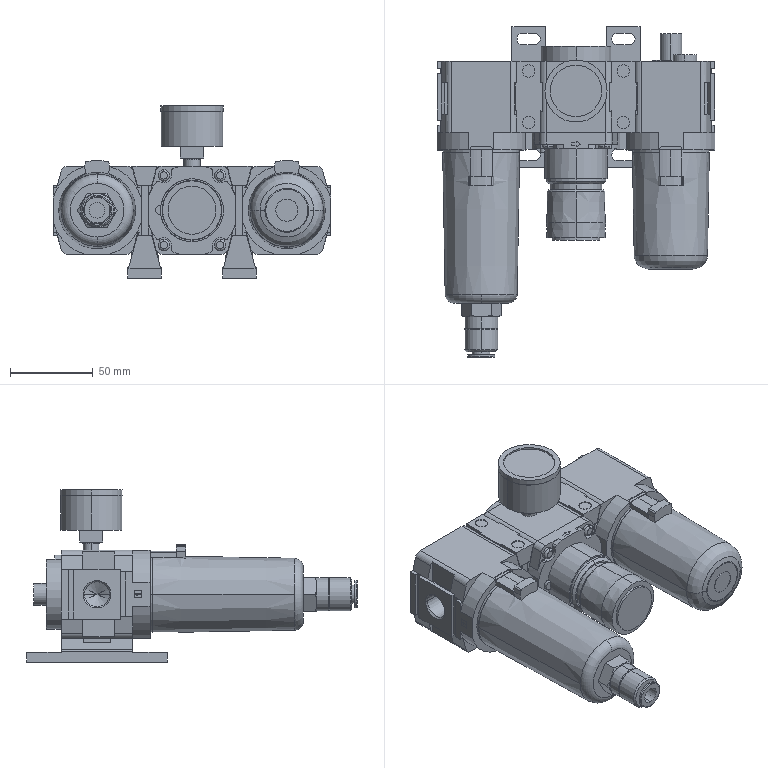Part | SolidWorks | features AEMSimFeature 1 | 15 solids | 967 faces | box 167.4 x 199.6 x 104 mm | volume 821277 mm3 | plane 672 | cylinder 209 | cone 62 | torus 24 | commonest cylinder face diameters 7 x20 8 x16 55 x16 14.95 x12 3 x10 7.5 x8